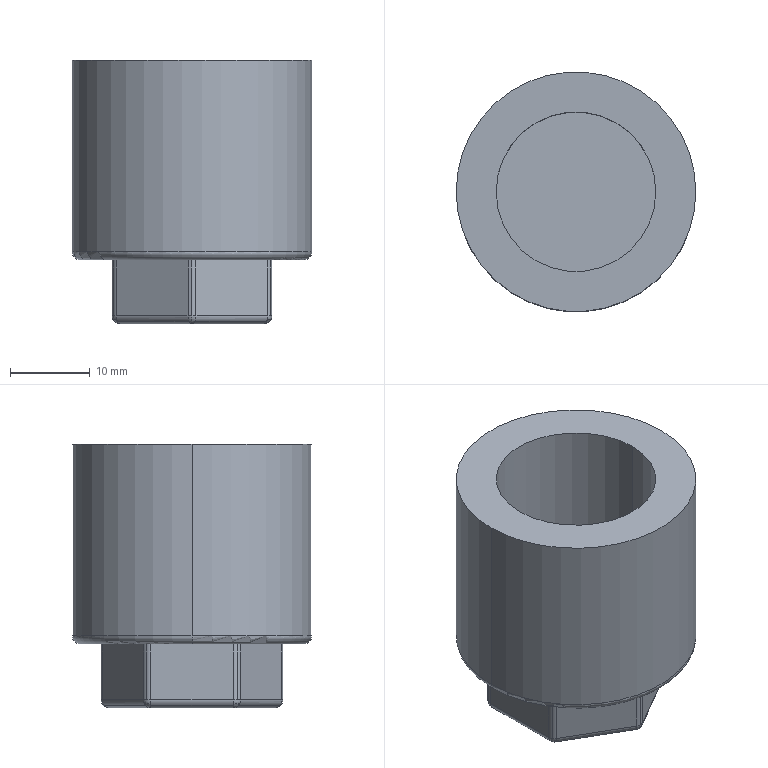Part | SolidWorks | features BaseBody 1 | 1 solid | 52 faces | box 30 x 30 x 33 mm | volume 14123 mm3 | cylinder 28 | sphere 12 | plane 10 | torus 2 | commonest cylinder face diameters 2 x24 20 x2 30 x2
STEP:
#1=CARTESIAN_POINT('',(0.,-10.392,-8.));
#2=VERTEX_POINT('',#1);
#3=CARTESIAN_POINT('',(-0.3536,-11.005,-7.707));
#4=VERTEX_POINT('',#3);
#5=CARTESIAN_POINT('',(0.,-10.392,-7.));
#6=DIRECTION('',(-0.866,0.5,0.));
#7=DIRECTION('',(0.,0.,-1.));
#8=AXIS2_PLACEMENT_3D('',#5,#6,#7);
#9=CIRCLE('',#8,1.);
#10=EDGE_CURVE('',#2,#4,#9,.T.);
#11=ORIENTED_EDGE('',*,*,#10,.F.);
#12=CARTESIAN_POINT('',(0.,-11.392,-7.));
#13=VERTEX_POINT('',#12);
#14=CARTESIAN_POINT('',(0.,-10.392,-7.));
#15=DIRECTION('',(-1.,0.,0.));
#16=DIRECTION('',(0.,-1.,0.));
#17=AXIS2_PLACEMENT_3D('',#14,#15,#16);
#18=CIRCLE('',#17,1.);
#19=EDGE_CURVE('',#2,#13,#18,.T.);
#20=ORIENTED_EDGE('',*,*,#19,.T.);
#21=CARTESIAN_POINT('',(-0.5,-11.258,-7.));
#22=VERTEX_POINT('',#21);
#23=CARTESIAN_POINT('',(0.,-10.392,-7.));
#24=DIRECTION('',(0.,0.,1.));
#25=DIRECTION('',(-0.5,-0.866,0.));
#26=AXIS2_PLACEMENT_3D('',#23,#24,#25);
#27=CIRCLE('',#26,1.);
#28=EDGE_CURVE('',#22,#13,#27,.T.);
#29=ORIENTED_EDGE('',*,*,#28,.F.);
#30=CARTESIAN_POINT('',(0.,-10.392,-7.));
#31=DIRECTION('',(-0.866,0.5,0.));
#32=DIRECTION('',(0.,0.,-1.));
#33=AXIS2_PLACEMENT_3D('',#30,#31,#32);
#34=CIRCLE('',#33,1.);
#35=EDGE_CURVE('',#4,#22,#34,.T.);
#36=ORIENTED_EDGE('',*,*,#35,.F.);
#37=EDGE_LOOP('',(#11,#20,#29,#36));
#38=FACE_OUTER_BOUND('',#37,.T.);
#39=CARTESIAN_POINT('',(0.,-10.392,-7.));
#40=DIRECTION('',(1.,0.,0.));
#41=DIRECTION('',(0.,-0.866,-0.5));
#42=AXIS2_PLACEMENT_3D('',#39,#40,#41);
#43=SPHERICAL_SURFACE('',#42,1.);
#44=ADVANCED_FACE('',(#38),#43,.T.);
#45=ORIENTED_EDGE('',*,*,#28,.T.);
#46=CARTESIAN_POINT('',(0.,-11.392,0.));
#47=VERTEX_POINT('',#46);
#48=CARTESIAN_POINT('',(0.,-11.392,0.));
#49=DIRECTION('',(0.,0.,1.));
#50=VECTOR('',#49,1000.);
#51=LINE('',#48,#50);
#52=EDGE_CURVE('',#13,#47,#51,.T.);
#53=ORIENTED_EDGE('',*,*,#52,.T.);
#54=CARTESIAN_POINT('',(-0.5,-11.258,0.));
#55=VERTEX_POINT('',#54);
#56=CARTESIAN_POINT('',(0.,-10.392,0.));
#57=DIRECTION('',(0.,0.,-1.));
#58=DIRECTION('',(0.,-1.,0.));
#59=AXIS2_PLACEMENT_3D('',#56,#57,#58);
#60=CIRCLE('',#59,1.);
#61=EDGE_CURVE('',#47,#55,#60,.T.);
#62=ORIENTED_EDGE('',*,*,#61,.T.);
#63=CARTESIAN_POINT('',(-0.5,-11.258,0.));
#64=DIRECTION('',(0.,0.,-1.));
#65=VECTOR('',#64,1000.);
#66=LINE('',#63,#65);
#67=EDGE_CURVE('',#55,#22,#66,.T.);
#68=ORIENTED_EDGE('',*,*,#67,.T.);
#69=EDGE_LOOP('',(#45,#53,#62,#68));
#70=FACE_OUTER_BOUND('',#69,.T.);
#71=CARTESIAN_POINT('',(0.,-10.392,0.));
#72=DIRECTION('',(0.,0.,1.));
#73=DIRECTION('',(0.,-1.,0.));
#74=AXIS2_PLACEMENT_3D('',#71,#72,#73);
#75=CYLINDRICAL_SURFACE('',#74,1.);
#76=ADVANCED_FACE('',(#70),#75,.T.);
#77=CARTESIAN_POINT('',(-9.447,-5.971,-7.447));
#78=VERTEX_POINT('',#77);
#79=CARTESIAN_POINT('',(-9.354,-5.809,-7.707));
#80=VERTEX_POINT('',#79);
#81=CARTESIAN_POINT('',(-9.,-5.196,-7.));
#82=DIRECTION('',(0.866,-0.5,0.));
#83=DIRECTION('',(-0.5,-0.866,0.));
#84=AXIS2_PLACEMENT_3D('',#81,#82,#83);
#85=CIRCLE('',#84,1.);
#86=EDGE_CURVE('',#78,#80,#85,.T.);
#87=ORIENTED_EDGE('',*,*,#86,.F.);
#88=CARTESIAN_POINT('',(-9.894,-5.196,-7.447));
#89=VERTEX_POINT('',#88);
#90=CARTESIAN_POINT('',(-9.,-5.196,-7.));
#91=DIRECTION('',(0.433,0.25,-0.866));
#92=DIRECTION('',(-0.8944,0.,-0.4472));
#93=AXIS2_PLACEMENT_3D('',#90,#91,#92);
#94=CIRCLE('',#93,1.);
#95=EDGE_CURVE('',#78,#89,#94,.T.);
#96=ORIENTED_EDGE('',*,*,#95,.T.);
#97=CARTESIAN_POINT('',(-9.707,-5.196,-7.707));
#98=VERTEX_POINT('',#97);
#99=CARTESIAN_POINT('',(-9.,-5.196,-7.));
#100=DIRECTION('',(0.,1.,0.));
#101=DIRECTION('',(0.,0.,-1.));
#102=AXIS2_PLACEMENT_3D('',#99,#100,#101);
#103=CIRCLE('',#102,1.);
#104=EDGE_CURVE('',#98,#89,#103,.T.);
#105=ORIENTED_EDGE('',*,*,#104,.F.);
#106=CARTESIAN_POINT('',(-9.,-5.196,-8.));
#107=VERTEX_POINT('',#106);
#108=CARTESIAN_POINT('',(-9.,-5.196,-7.));
#109=DIRECTION('',(0.,1.,0.));
#110=DIRECTION('',(0.,0.,-1.));
#111=AXIS2_PLACEMENT_3D('',#108,#109,#110);
#112=CIRCLE('',#111,1.);
#113=EDGE_CURVE('',#107,#98,#112,.T.);
#114=ORIENTED_EDGE('',*,*,#113,.F.);
#115=CARTESIAN_POINT('',(-9.,-5.196,-7.));
#116=DIRECTION('',(0.866,-0.5,0.));
#117=DIRECTION('',(-0.5,-0.866,0.));
#118=AXIS2_PLACEMENT_3D('',#115,#116,#117);
#119=CIRCLE('',#118,1.);
#120=EDGE_CURVE('',#80,#107,#119,.T.);
#121=ORIENTED_EDGE('',*,*,#120,.F.);
#122=EDGE_LOOP('',(#87,#96,#105,#114,#121));
#123=FACE_OUTER_BOUND('',#122,.T.);
#124=CARTESIAN_POINT('',(-9.,-5.196,-7.));
#125=DIRECTION('',(-0.433,-0.25,0.866));
#126=DIRECTION('',(-0.75,-0.433,-0.5));
#127=AXIS2_PLACEMENT_3D('',#124,#125,#126);
#128=SPHERICAL_SURFACE('',#127,1.);
#129=ADVANCED_FACE('',(#123),#128,.T.);
#130=CARTESIAN_POINT('',(-10.,-5.196,-7.));
#131=VERTEX_POINT('',#130);
#132=CARTESIAN_POINT('',(-9.866,-5.696,-7.));
#133=VERTEX_POINT('',#132);
#134=CARTESIAN_POINT('',(-9.,-5.196,-7.));
#135=DIRECTION('',(0.,0.,1.));
#136=DIRECTION('',(-1.,0.,0.));
#137=AXIS2_PLACEMENT_3D('',#134,#135,#136);
#138=CIRCLE('',#137,1.);
#139=EDGE_CURVE('',#131,#133,#138,.T.);
#140=ORIENTED_EDGE('',*,*,#139,.T.);
#141=CARTESIAN_POINT('',(-9.866,-5.696,0.));
#142=VERTEX_POINT('',#141);
#143=CARTESIAN_POINT('',(-9.866,-5.696,0.));
#144=DIRECTION('',(0.,0.,1.));
#145=VECTOR('',#144,1000.);
#146=LINE('',#143,#145);
#147=EDGE_CURVE('',#133,#142,#146,.T.);
#148=ORIENTED_EDGE('',*,*,#147,.T.);
#149=CARTESIAN_POINT('',(-10.,-5.196,0.));
#150=VERTEX_POINT('',#149);
#151=CARTESIAN_POINT('',(-9.,-5.196,0.));
#152=DIRECTION('',(0.,0.,-1.));
#153=DIRECTION('',(-0.866,-0.5,0.));
#154=AXIS2_PLACEMENT_3D('',#151,#152,#153);
#155=CIRCLE('',#154,1.);
#156=EDGE_CURVE('',#142,#150,#155,.T.);
#157=ORIENTED_EDGE('',*,*,#156,.T.);
#158=CARTESIAN_POINT('',(-10.,-5.196,0.));
#159=DIRECTION('',(0.,0.,-1.));
#160=VECTOR('',#159,1000.);
#161=LINE('',#158,#160);
#162=EDGE_CURVE('',#150,#131,#161,.T.);
#163=ORIENTED_EDGE('',*,*,#162,.T.);
#164=EDGE_LOOP('',(#140,#148,#157,#163));
#165=FACE_OUTER_BOUND('',#164,.T.);
#166=CARTESIAN_POINT('',(-9.,-5.196,0.));
#167=DIRECTION('',(0.,0.,1.));
#168=DIRECTION('',(-0.866,-0.5,0.));
#169=AXIS2_PLACEMENT_3D('',#166,#167,#168);
#170=CYLINDRICAL_SURFACE('',#169,1.);
#171=ADVANCED_FACE('',(#165),#170,.T.);
#172=CARTESIAN_POINT('',(9.894,-5.196,-7.447));
#173=VERTEX_POINT('',#172);
#174=CARTESIAN_POINT('',(9.707,-5.196,-7.707));
#175=VERTEX_POINT('',#174);
#176=CARTESIAN_POINT('',(9.,-5.196,-7.));
#177=DIRECTION('',(0.,1.,0.));
#178=DIRECTION('',(1.,0.,0.));
#179=AXIS2_PLACEMENT_3D('',#176,#177,#178);
#180=CIRCLE('',#179,1.);
#181=EDGE_CURVE('',#173,#175,#180,.T.);
#182=ORIENTED_EDGE('',*,*,#181,.F.);
#183=CARTESIAN_POINT('',(9.447,-5.971,-7.447));
#184=VERTEX_POINT('',#183);
#185=CARTESIAN_POINT('',(9.,-5.196,-7.));
#186=DIRECTION('',(-0.433,0.25,-0.866));
#187=DIRECTION('',(-0.8944,0.,0.4472));
#188=AXIS2_PLACEMENT_3D('',#185,#186,#187);
#189=CIRCLE('',#188,1.);
#190=EDGE_CURVE('',#173,#184,#189,.T.);
#191=ORIENTED_EDGE('',*,*,#190,.T.);
#192=CARTESIAN_POINT('',(9.354,-5.809,-7.707));
#193=VERTEX_POINT('',#192);
#194=CARTESIAN_POINT('',(9.,-5.196,-7.));
#195=DIRECTION('',(-0.866,-0.5,0.));
#196=DIRECTION('',(0.,0.,-1.));
#197=AXIS2_PLACEMENT_3D('',#194,#195,#196);
#198=CIRCLE('',#197,1.);
#199=EDGE_CURVE('',#193,#184,#198,.T.);
#200=ORIENTED_EDGE('',*,*,#199,.F.);
#201=CARTESIAN_POINT('',(9.,-5.196,-8.));
#202=VERTEX_POINT('',#201);
#203=CARTESIAN_POINT('',(9.,-5.196,-7.));
#204=DIRECTION('',(-0.866,-0.5,0.));
#205=DIRECTION('',(0.,0.,-1.));
#206=AXIS2_PLACEMENT_3D('',#203,#204,#205);
#207=CIRCLE('',#206,1.);
#208=EDGE_CURVE('',#202,#193,#207,.T.);
#209=ORIENTED_EDGE('',*,*,#208,.F.);
#210=CARTESIAN_POINT('',(9.,-5.196,-7.));
#211=DIRECTION('',(0.,1.,0.));
#212=DIRECTION('',(1.,0.,0.));
#213=AXIS2_PLACEMENT_3D('',#210,#211,#212);
#214=CIRCLE('',#213,1.);
#215=EDGE_CURVE('',#175,#202,#214,.T.);
#216=ORIENTED_EDGE('',*,*,#215,.F.);
#217=EDGE_LOOP('',(#182,#191,#200,#209,#216));
#218=FACE_OUTER_BOUND('',#217,.T.);
#219=CARTESIAN_POINT('',(9.,-5.196,-7.));
#220=DIRECTION('',(0.433,-0.25,0.866));
#221=DIRECTION('',(0.75,-0.433,-0.5));
#222=AXIS2_PLACEMENT_3D('',#219,#220,#221);
#223=SPHERICAL_SURFACE('',#222,1.);
#224=ADVANCED_FACE('',(#218),#223,.T.);
#225=CARTESIAN_POINT('',(9.5,-6.062,-7.));
#226=VERTEX_POINT('',#225);
#227=CARTESIAN_POINT('',(9.866,-5.696,-7.));
#228=VERTEX_POINT('',#227);
#229=CARTESIAN_POINT('',(9.,-5.196,-7.));
#230=DIRECTION('',(0.,0.,1.));
#231=DIRECTION('',(0.5,-0.866,0.));
#232=AXIS2_PLACEMENT_3D('',#229,#230,#231);
#233=CIRCLE('',#232,1.);
#234=EDGE_CURVE('',#226,#228,#233,.T.);
#235=ORIENTED_EDGE('',*,*,#234,.T.);
#236=CARTESIAN_POINT('',(9.866,-5.696,0.));
#237=VERTEX_POINT('',#236);
#238=CARTESIAN_POINT('',(9.866,-5.696,0.));
#239=DIRECTION('',(0.,0.,1.));
#240=VECTOR('',#239,1000.);
#241=LINE('',#238,#240);
#242=EDGE_CURVE('',#228,#237,#241,.T.);
#243=ORIENTED_EDGE('',*,*,#242,.T.);
#244=CARTESIAN_POINT('',(9.5,-6.062,0.));
#245=VERTEX_POINT('',#244);
#246=CARTESIAN_POINT('',(9.,-5.196,0.));
#247=DIRECTION('',(0.,0.,-1.));
#248=DIRECTION('',(0.866,-0.5,0.));
#249=AXIS2_PLACEMENT_3D('',#246,#247,#248);
#250=CIRCLE('',#249,1.);
#251=EDGE_CURVE('',#237,#245,#250,.T.);
#252=ORIENTED_EDGE('',*,*,#251,.T.);
#253=CARTESIAN_POINT('',(9.5,-6.062,0.));
#254=DIRECTION('',(0.,0.,-1.));
#255=VECTOR('',#254,1000.);
#256=LINE('',#253,#255);
#257=EDGE_CURVE('',#245,#226,#256,.T.);
#258=ORIENTED_EDGE('',*,*,#257,.T.);
#259=EDGE_LOOP('',(#235,#243,#252,#258));
#260=FACE_OUTER_BOUND('',#259,.T.);
#261=CARTESIAN_POINT('',(9.,-5.196,0.));
#262=DIRECTION('',(0.,0.,1.));
#263=DIRECTION('',(0.866,-0.5,0.));
#264=AXIS2_PLACEMENT_3D('',#261,#262,#263);
#265=CYLINDRICAL_SURFACE('',#264,1.);
#266=ADVANCED_FACE('',(#260),#265,.T.);
#267=CARTESIAN_POINT('',(0.5,-11.258,-7.));
#268=VERTEX_POINT('',#267);
#269=CARTESIAN_POINT('',(0.3536,-11.005,-7.707));
#270=VERTEX_POINT('',#269);
#271=CARTESIAN_POINT('',(0.,-10.392,-7.));
#272=DIRECTION('',(0.866,0.5,0.));
#273=DIRECTION('',(0.5,-0.866,0.));
#274=AXIS2_PLACEMENT_3D('',#271,#272,#273);
#275=CIRCLE('',#274,1.);
#276=EDGE_CURVE('',#268,#270,#275,.T.);
#277=ORIENTED_EDGE('',*,*,#276,.T.);
#278=CARTESIAN_POINT('',(7.354,-6.963,-7.707));
#279=DIRECTION('',(0.866,0.5,0.));
#280=VECTOR('',#279,1000.);
#281=LINE('',#278,#280);
#282=EDGE_CURVE('',#270,#193,#281,.T.);
#283=ORIENTED_EDGE('',*,*,#282,.T.);
#284=ORIENTED_EDGE('',*,*,#199,.T.);
#285=CARTESIAN_POINT('',(9.,-5.196,-7.));
#286=DIRECTION('',(-0.866,-0.5,0.));
#287=DIRECTION('',(0.,0.,-1.));
#288=AXIS2_PLACEMENT_3D('',#285,#286,#287);
#289=CIRCLE('',#288,1.);
#290=EDGE_CURVE('',#184,#226,#289,.T.);
#291=ORIENTED_EDGE('',*,*,#290,.T.);
#292=CARTESIAN_POINT('',(7.5,-7.217,-7.));
#293=DIRECTION('',(-0.866,-0.5,0.));
#294=VECTOR('',#293,1000.);
#295=LINE('',#292,#294);
#296=EDGE_CURVE('',#226,#268,#295,.T.);
#297=ORIENTED_EDGE('',*,*,#296,.T.);
#298=EDGE_LOOP('',(#277,#283,#284,#291,#297));
#299=FACE_OUTER_BOUND('',#298,.T.);
#300=CARTESIAN_POINT('',(7.,-6.351,-7.));
#301=DIRECTION('',(0.866,0.5,0.));
#302=DIRECTION('',(0.3536,-0.6124,-0.7071));
#303=AXIS2_PLACEMENT_3D('',#300,#301,#302);
#304=CYLINDRICAL_SURFACE('',#303,1.);
#305=ADVANCED_FACE('',(#299),#304,.T.);
#306=CARTESIAN_POINT('',(-9.894,5.196,-7.447));
#307=VERTEX_POINT('',#306);
#308=CARTESIAN_POINT('',(-9.707,5.196,-7.707));
#309=VERTEX_POINT('',#308);
#310=CARTESIAN_POINT('',(-9.,5.196,-7.));
#311=DIRECTION('',(0.,-1.,0.));
#312=DIRECTION('',(-1.,0.,0.));
#313=AXIS2_PLACEMENT_3D('',#310,#311,#312);
#314=CIRCLE('',#313,1.);
#315=EDGE_CURVE('',#307,#309,#314,.T.);
#316=ORIENTED_EDGE('',*,*,#315,.F.);
#317=CARTESIAN_POINT('',(-9.447,5.971,-7.447));
#318=VERTEX_POINT('',#317);
#319=CARTESIAN_POINT('',(-9.,5.196,-7.));
#320=DIRECTION('',(0.433,-0.25,-0.866));
#321=DIRECTION('',(-0.8944,0.,-0.4472));
#322=AXIS2_PLACEMENT_3D('',#319,#320,#321);
#323=CIRCLE('',#322,1.);
#324=EDGE_CURVE('',#307,#318,#323,.T.);
#325=ORIENTED_EDGE('',*,*,#324,.T.);
#326=CARTESIAN_POINT('',(-9.354,5.809,-7.707));
#327=VERTEX_POINT('',#326);
#328=CARTESIAN_POINT('',(-9.,5.196,-7.));
#329=DIRECTION('',(0.866,0.5,0.));
#330=DIRECTION('',(0.,0.,-1.));
#331=AXIS2_PLACEMENT_3D('',#328,#329,#330);
#332=CIRCLE('',#331,1.);
#333=EDGE_CURVE('',#327,#318,#332,.T.);
#334=ORIENTED_EDGE('',*,*,#333,.F.);
#335=CARTESIAN_POINT('',(-9.,5.196,-8.));
#336=VERTEX_POINT('',#335);
#337=CARTESIAN_POINT('',(-9.,5.196,-7.));
#338=DIRECTION('',(0.866,0.5,0.));
#339=DIRECTION('',(0.,0.,-1.));
#340=AXIS2_PLACEMENT_3D('',#337,#338,#339);
#341=CIRCLE('',#340,1.);
#342=EDGE_CURVE('',#336,#327,#341,.T.);
#343=ORIENTED_EDGE('',*,*,#342,.F.);
#344=CARTESIAN_POINT('',(-9.,5.196,-7.));
#345=DIRECTION('',(0.,-1.,0.));
#346=DIRECTION('',(-1.,0.,0.));
#347=AXIS2_PLACEMENT_3D('',#344,#345,#346);
#348=CIRCLE('',#347,1.);
#349=EDGE_CURVE('',#309,#336,#348,.T.);
#350=ORIENTED_EDGE('',*,*,#349,.F.);
#351=EDGE_LOOP('',(#316,#325,#334,#343,#350));
#352=FACE_OUTER_BOUND('',#351,.T.);
#353=CARTESIAN_POINT('',(-9.,5.196,-7.));
#354=DIRECTION('',(-0.433,0.25,0.866));
#355=DIRECTION('',(-0.75,0.433,-0.5));
#356=AXIS2_PLACEMENT_3D('',#353,#354,#355);
#357=SPHERICAL_SURFACE('',#356,1.);
#358=ADVANCED_FACE('',(#352),#357,.T.);
#359=CARTESIAN_POINT('',(-9.5,6.062,-7.));
#360=VERTEX_POINT('',#359);
#361=CARTESIAN_POINT('',(-9.866,5.696,-7.));
#362=VERTEX_POINT('',#361);
#363=CARTESIAN_POINT('',(-9.,5.196,-7.));
#364=DIRECTION('',(0.,0.,1.));
#365=DIRECTION('',(-0.5,0.866,0.));
#366=AXIS2_PLACEMENT_3D('',#363,#364,#365);
#367=CIRCLE('',#366,1.);
#368=EDGE_CURVE('',#360,#362,#367,.T.);
#369=ORIENTED_EDGE('',*,*,#368,.T.);
#370=CARTESIAN_POINT('',(-9.866,5.696,0.));
#371=VERTEX_POINT('',#370);
#372=CARTESIAN_POINT('',(-9.866,5.696,0.));
#373=DIRECTION('',(0.,0.,1.));
#374=VECTOR('',#373,1000.);
#375=LINE('',#372,#374);
#376=EDGE_CURVE('',#362,#371,#375,.T.);
#377=ORIENTED_EDGE('',*,*,#376,.T.);
#378=CARTESIAN_POINT('',(-9.5,6.062,0.));
#379=VERTEX_POINT('',#378);
#380=CARTESIAN_POINT('',(-9.,5.196,0.));
#381=DIRECTION('',(0.,0.,-1.));
#382=DIRECTION('',(-0.866,0.5,0.));
#383=AXIS2_PLACEMENT_3D('',#380,#381,#382);
#384=CIRCLE('',#383,1.);
#385=EDGE_CURVE('',#371,#379,#384,.T.);
#386=ORIENTED_EDGE('',*,*,#385,.T.);
#387=CARTESIAN_POINT('',(-9.5,6.062,0.));
#388=DIRECTION('',(0.,0.,-1.));
#389=VECTOR('',#388,1000.);
#390=LINE('',#387,#389);
#391=EDGE_CURVE('',#379,#360,#390,.T.);
#392=ORIENTED_EDGE('',*,*,#391,.T.);
#393=EDGE_LOOP('',(#369,#377,#386,#392));
#394=FACE_OUTER_BOUND('',#393,.T.);
#395=CARTESIAN_POINT('',(-9.,5.196,0.));
#396=DIRECTION('',(0.,0.,1.));
#397=DIRECTION('',(-0.866,0.5,0.));
#398=AXIS2_PLACEMENT_3D('',#395,#396,#397);
#399=CYLINDRICAL_SURFACE('',#398,1.);
#400=ADVANCED_FACE('',(#394),#399,.T.);
#401=CARTESIAN_POINT('',(9.447,5.971,-7.447));
#402=VERTEX_POINT('',#401);
#403=CARTESIAN_POINT('',(9.354,5.809,-7.707));
#404=VERTEX_POINT('',#403);
#405=CARTESIAN_POINT('',(9.,5.196,-7.));
#406=DIRECTION('',(-0.866,0.5,0.));
#407=DIRECTION('',(0.5,0.866,0.));
#408=AXIS2_PLACEMENT_3D('',#405,#406,#407);
#409=CIRCLE('',#408,1.);
#410=EDGE_CURVE('',#402,#404,#409,.T.);
#411=ORIENTED_EDGE('',*,*,#410,.F.);
#412=CARTESIAN_POINT('',(9.894,5.196,-7.447));
#413=VERTEX_POINT('',#412);
#414=CARTESIAN_POINT('',(9.,5.196,-7.));
#415=DIRECTION('',(-0.433,-0.25,-0.866));
#416=DIRECTION('',(-0.8944,0.,0.4472));
#417=AXIS2_PLACEMENT_3D('',#414,#415,#416);
#418=CIRCLE('',#417,1.);
#419=EDGE_CURVE('',#402,#413,#418,.T.);
#420=ORIENTED_EDGE('',*,*,#419,.T.);
#421=CARTESIAN_POINT('',(9.707,5.196,-7.707));
#422=VERTEX_POINT('',#421);
#423=CARTESIAN_POINT('',(9.,5.196,-7.));
#424=DIRECTION('',(0.,-1.,0.));
#425=DIRECTION('',(0.,0.,-1.));
#426=AXIS2_PLACEMENT_3D('',#423,#424,#425);
#427=CIRCLE('',#426,1.);
#428=EDGE_CURVE('',#422,#413,#427,.T.);
#429=ORIENTED_EDGE('',*,*,#428,.F.);
#430=CARTESIAN_POINT('',(9.,5.196,-8.));
#431=VERTEX_POINT('',#430);
#432=CARTESIAN_POINT('',(9.,5.196,-7.));
#433=DIRECTION('',(0.,-1.,0.));
#434=DIRECTION('',(0.,0.,-1.));
#435=AXIS2_PLACEMENT_3D('',#432,#433,#434);
#436=CIRCLE('',#435,1.);
#437=EDGE_CURVE('',#431,#422,#436,.T.);
#438=ORIENTED_EDGE('',*,*,#437,.F.);
#439=CARTESIAN_POINT('',(9.,5.196,-7.));
#440=DIRECTION('',(-0.866,0.5,0.));
#441=DIRECTION('',(0.5,0.866,0.));
#442=AXIS2_PLACEMENT_3D('',#439,#440,#441);
#443=CIRCLE('',#442,1.);
#444=EDGE_CURVE('',#404,#431,#443,.T.);
#445=ORIENTED_EDGE('',*,*,#444,.F.);
#446=EDGE_LOOP('',(#411,#420,#429,#438,#445));
#447=FACE_OUTER_BOUND('',#446,.T.);
#448=CARTESIAN_POINT('',(9.,5.196,-7.));
#449=DIRECTION('',(0.433,0.25,0.866));
#450=DIRECTION('',(0.75,0.433,-0.5));
#451=AXIS2_PLACEMENT_3D('',#448,#449,#450);
#452=SPHERICAL_SURFACE('',#451,1.);
#453=ADVANCED_FACE('',(#447),#452,.T.);
#454=CARTESIAN_POINT('',(10.,5.196,-7.));
#455=VERTEX_POINT('',#454);
#456=CARTESIAN_POINT('',(9.866,5.696,-7.));
#457=VERTEX_POINT('',#456);
#458=CARTESIAN_POINT('',(9.,5.196,-7.));
#459=DIRECTION('',(0.,0.,1.));
#460=DIRECTION('',(1.,0.,0.));
#461=AXIS2_PLACEMENT_3D('',#458,#459,#460);
#462=CIRCLE('',#461,1.);
#463=EDGE_CURVE('',#455,#457,#462,.T.);
#464=ORIENTED_EDGE('',*,*,#463,.T.);
#465=CARTESIAN_POINT('',(9.866,5.696,0.));
#466=VERTEX_POINT('',#465);
#467=CARTESIAN_POINT('',(9.866,5.696,0.));
#468=DIRECTION('',(0.,0.,1.));
#469=VECTOR('',#468,1000.);
#470=LINE('',#467,#469);
#471=EDGE_CURVE('',#457,#466,#470,.T.);
#472=ORIENTED_EDGE('',*,*,#471,.T.);
#473=CARTESIAN_POINT('',(10.,5.196,0.));
#474=VERTEX_POINT('',#473);
#475=CARTESIAN_POINT('',(9.,5.196,0.));
#476=DIRECTION('',(0.,0.,-1.));
#477=DIRECTION('',(0.866,0.5,0.));
#478=AXIS2_PLACEMENT_3D('',#475,#476,#477);
#479=CIRCLE('',#478,1.);
#480=EDGE_CURVE('',#466,#474,#479,.T.);
#481=ORIENTED_EDGE('',*,*,#480,.T.);
#482=CARTESIAN_POINT('',(10.,5.196,0.));
#483=DIRECTION('',(0.,0.,-1.));
#484=VECTOR('',#483,1000.);
#485=LINE('',#482,#484);
#486=EDGE_CURVE('',#474,#455,#485,.T.);
#487=ORIENTED_EDGE('',*,*,#486,.T.);
#488=EDGE_LOOP('',(#464,#472,#481,#487));
#489=FACE_OUTER_BOUND('',#488,.T.);
#490=CARTESIAN_POINT('',(9.,5.196,0.));
#491=DIRECTION('',(0.,0.,1.));
#492=DIRECTION('',(0.866,0.5,0.));
#493=AXIS2_PLACEMENT_3D('',#490,#491,#492);
#494=CYLINDRICAL_SURFACE('',#493,1.);
#495=ADVANCED_FACE('',(#489),#494,.T.);
#496=CARTESIAN_POINT('',(10.,-5.196,-7.));
#497=VERTEX_POINT('',#496);
#498=CARTESIAN_POINT('',(9.,-5.196,-7.));
#499=DIRECTION('',(0.,1.,0.));
#500=DIRECTION('',(1.,0.,0.));
#501=AXIS2_PLACEMENT_3D('',#498,#499,#500);
#502=CIRCLE('',#501,1.);
#503=EDGE_CURVE('',#497,#173,#502,.T.);
#504=ORIENTED_EDGE('',*,*,#503,.T.);
#505=ORIENTED_EDGE('',*,*,#181,.T.);
#506=CARTESIAN_POINT('',(9.707,2.887,-7.707));
#507=DIRECTION('',(0.,1.,0.));
#508=VECTOR('',#507,1000.);
#509=LINE('',#506,#508);
#510=EDGE_CURVE('',#175,#422,#509,.T.);
#511=ORIENTED_EDGE('',*,*,#510,.T.);
#512=ORIENTED_EDGE('',*,*,#428,.T.);
#513=CARTESIAN_POINT('',(9.,5.196,-7.));
#514=DIRECTION('',(0.,-1.,0.));
#515=DIRECTION('',(0.,0.,-1.));
#516=AXIS2_PLACEMENT_3D('',#513,#514,#515);
#517=CIRCLE('',#516,1.);
#518=EDGE_CURVE('',#413,#455,#517,.T.);
#519=ORIENTED_EDGE('',*,*,#518,.T.);
#520=CARTESIAN_POINT('',(10.,2.887,-7.));
#521=DIRECTION('',(0.,-1.,0.));
#522=VECTOR('',#521,1000.);
#523=LINE('',#520,#522);
#524=EDGE_CURVE('',#455,#497,#523,.T.);
#525=ORIENTED_EDGE('',*,*,#524,.T.);
#526=EDGE_LOOP('',(#504,#505,#511,#512,#519,#525));
#527=FACE_OUTER_BOUND('',#526,.T.);
#528=CARTESIAN_POINT('',(9.,2.887,-7.));
#529=DIRECTION('',(0.,1.,0.));
#530=DIRECTION('',(0.7071,0.,-0.7071));
#531=AXIS2_PLACEMENT_3D('',#528,#529,#530);
#532=CYLINDRICAL_SURFACE('',#531,1.);
#533=ADVANCED_FACE('',(#527),#532,.T.);
#534=CARTESIAN_POINT('',(0.,11.392,-7.));
#535=VERTEX_POINT('',#534);
#536=CARTESIAN_POINT('',(-0.5,11.258,-7.));
#537=VERTEX_POINT('',#536);
#538=CARTESIAN_POINT('',(0.,10.392,-7.));
#539=DIRECTION('',(0.,0.,1.));
#540=DIRECTION('',(0.5,0.866,0.));
#541=AXIS2_PLACEMENT_3D('',#538,#539,#540);
#542=CIRCLE('',#541,1.);
#543=EDGE_CURVE('',#535,#537,#542,.T.);
#544=ORIENTED_EDGE('',*,*,#543,.F.);
#545=CARTESIAN_POINT('',(0.,10.392,-8.));
#546=VERTEX_POINT('',#545);
#547=CARTESIAN_POINT('',(0.,10.392,-7.));
#548=DIRECTION('',(-1.,0.,0.));
#549=DIRECTION('',(0.,-1.,0.));
#550=AXIS2_PLACEMENT_3D('',#547,#548,#549);
#551=CIRCLE('',#550,1.);
#552=EDGE_CURVE('',#535,#546,#551,.T.);
#553=ORIENTED_EDGE('',*,*,#552,.T.);
#554=CARTESIAN_POINT('',(-0.3536,11.005,-7.707));
#555=VERTEX_POINT('',#554);
#556=CARTESIAN_POINT('',(0.,10.392,-7.));
#557=DIRECTION('',(-0.866,-0.5,0.));
#558=DIRECTION('',(-0.5,0.866,0.));
#559=AXIS2_PLACEMENT_3D('',#556,#557,#558);
#560=CIRCLE('',#559,1.);
#561=EDGE_CURVE('',#555,#546,#560,.T.);
#562=ORIENTED_EDGE('',*,*,#561,.F.);
#563=CARTESIAN_POINT('',(0.,10.392,-7.));
#564=DIRECTION('',(-0.866,-0.5,0.));
#565=DIRECTION('',(-0.5,0.866,0.));
#566=AXIS2_PLACEMENT_3D('',#563,#564,#565);
#567=CIRCLE('',#566,1.);
#568=EDGE_CURVE('',#537,#555,#567,.T.);
#569=ORIENTED_EDGE('',*,*,#568,.F.);
#570=EDGE_LOOP('',(#544,#553,#562,#569));
#571=FACE_OUTER_BOUND('',#570,.T.);
#572=CARTESIAN_POINT('',(0.,10.392,-7.));
#573=DIRECTION('',(1.,0.,0.));
#574=DIRECTION('',(0.,0.866,-0.5));
#575=AXIS2_PLACEMENT_3D('',#572,#573,#574);
#576=SPHERICAL_SURFACE('',#575,1.);
#577=ADVANCED_FACE('',(#571),#576,.T.);
#578=CARTESIAN_POINT('',(0.5,11.258,-7.));
#579=VERTEX_POINT('',#578);
#580=CARTESIAN_POINT('',(0.,10.392,-7.));
#581=DIRECTION('',(0.,0.,1.));
#582=DIRECTION('',(0.5,0.866,0.));
#583=AXIS2_PLACEMENT_3D('',#580,#581,#582);
#584=CIRCLE('',#583,1.);
#585=EDGE_CURVE('',#579,#535,#584,.T.);
#586=ORIENTED_EDGE('',*,*,#585,.T.);
#587=CARTESIAN_POINT('',(0.,11.392,0.));
#588=VERTEX_POINT('',#587);
#589=CARTESIAN_POINT('',(0.,11.392,0.));
#590=DIRECTION('',(0.,0.,1.));
#591=VECTOR('',#590,1000.);
#592=LINE('',#589,#591);
#593=EDGE_CURVE('',#535,#588,#592,.T.);
#594=ORIENTED_EDGE('',*,*,#593,.T.);
#595=CARTESIAN_POINT('',(0.5,11.258,0.));
#596=VERTEX_POINT('',#595);
#597=CARTESIAN_POINT('',(0.,10.392,0.));
#598=DIRECTION('',(0.,0.,-1.));
#599=DIRECTION('',(0.,1.,0.));
#600=AXIS2_PLACEMENT_3D('',#597,#598,#599);
#601=CIRCLE('',#600,1.);
#602=EDGE_CURVE('',#588,#596,#601,.T.);
#603=ORIENTED_EDGE('',*,*,#602,.T.);
#604=CARTESIAN_POINT('',(0.5,11.258,0.));
#605=DIRECTION('',(0.,0.,-1.));
#606=VECTOR('',#605,1000.);
#607=LINE('',#604,#606);
#608=EDGE_CURVE('',#596,#579,#607,.T.);
#609=ORIENTED_EDGE('',*,*,#608,.T.);
#610=EDGE_LOOP('',(#586,#594,#603,#609));
#611=FACE_OUTER_BOUND('',#610,.T.);
#612=CARTESIAN_POINT('',(0.,10.392,0.));
#613=DIRECTION('',(0.,0.,1.));
#614=DIRECTION('',(0.,1.,0.));
#615=AXIS2_PLACEMENT_3D('',#612,#613,#614);
#616=CYLINDRICAL_SURFACE('',#615,1.);
#617=ADVANCED_FACE('',(#611),#616,.T.);
#618=CARTESIAN_POINT('',(9.5,6.062,-7.));
#619=VERTEX_POINT('',#618);
#620=CARTESIAN_POINT('',(9.,5.196,-7.));
#621=DIRECTION('',(-0.866,0.5,0.));
#622=DIRECTION('',(0.5,0.866,0.));
#623=AXIS2_PLACEMENT_3D('',#620,#621,#622);
#624=CIRCLE('',#623,1.);
#625=EDGE_CURVE('',#619,#402,#624,.T.);
#626=ORIENTED_EDGE('',*,*,#625,.T.);
#627=ORIENTED_EDGE('',*,*,#410,.T.);
#628=CARTESIAN_POINT('',(0.3536,11.005,-7.707));
#629=VERTEX_POINT('',#628);
#630=CARTESIAN_POINT('',(2.354,9.85,-7.707));
#631=DIRECTION('',(-0.866,0.5,0.));
#632=VECTOR('',#631,1000.);
#633=LINE('',#630,#632);
#634=EDGE_CURVE('',#404,#629,#633,.T.);
#635=ORIENTED_EDGE('',*,*,#634,.T.);
#636=CARTESIAN_POINT('',(0.,10.392,-7.));
#637=DIRECTION('',(0.866,-0.5,0.));
#638=DIRECTION('',(0.,0.,-1.));
#639=AXIS2_PLACEMENT_3D('',#636,#637,#638);
#640=CIRCLE('',#639,1.);
#641=EDGE_CURVE('',#629,#579,#640,.T.);
#642=ORIENTED_EDGE('',*,*,#641,.T.);
#643=CARTESIAN_POINT('',(2.5,10.104,-7.));
#644=DIRECTION('',(0.866,-0.5,0.));
#645=VECTOR('',#644,1000.);
#646=LINE('',#643,#645);
#647=EDGE_CURVE('',#579,#619,#646,.T.);
#648=ORIENTED_EDGE('',*,*,#647,.T.);
#649=EDGE_LOOP('',(#626,#627,#635,#642,#648));
#650=FACE_OUTER_BOUND('',#649,.T.);
#651=CARTESIAN_POINT('',(2.,9.238,-7.));
#652=DIRECTION('',(-0.866,0.5,0.));
#653=DIRECTION('',(0.3536,0.6124,-0.7071));
#654=AXIS2_PLACEMENT_3D('',#651,#652,#653);
#655=CYLINDRICAL_SURFACE('',#654,1.);
#656=ADVANCED_FACE('',(#650),#655,.T.);
#657=ORIENTED_EDGE('',*,*,#568,.T.);
#658=CARTESIAN_POINT('',(-7.354,6.963,-7.707));
#659=DIRECTION('',(-0.866,-0.5,0.));
#660=VECTOR('',#659,1000.);
#661=LINE('',#658,#660);
#662=EDGE_CURVE('',#555,#327,#661,.T.);
#663=ORIENTED_EDGE('',*,*,#662,.T.);
#664=ORIENTED_EDGE('',*,*,#333,.T.);
#665=CARTESIAN_POINT('',(-9.,5.196,-7.));
#666=DIRECTION('',(0.866,0.5,0.));
#667=DIRECTION('',(0.,0.,-1.));
#668=AXIS2_PLACEMENT_3D('',#665,#666,#667);
#669=CIRCLE('',#668,1.);
#670=EDGE_CURVE('',#318,#360,#669,.T.);
#671=ORIENTED_EDGE('',*,*,#670,.T.);
#672=CARTESIAN_POINT('',(-7.5,7.217,-7.));
#673=DIRECTION('',(0.866,0.5,0.));
#674=VECTOR('',#673,1000.);
#675=LINE('',#672,#674);
#676=EDGE_CURVE('',#360,#537,#675,.T.);
#677=ORIENTED_EDGE('',*,*,#676,.T.);
#678=EDGE_LOOP('',(#657,#663,#664,#671,#677));
#679=FACE_OUTER_BOUND('',#678,.T.);
#680=CARTESIAN_POINT('',(-7.,6.351,-7.));
#681=DIRECTION('',(-0.866,-0.5,0.));
#682=DIRECTION('',(-0.3536,0.6124,-0.7071));
#683=AXIS2_PLACEMENT_3D('',#680,#681,#682);
#684=CYLINDRICAL_SURFACE('',#683,1.);
#685=ADVANCED_FACE('',(#679),#684,.T.);
#686=CARTESIAN_POINT('',(-10.,5.196,-7.));
#687=VERTEX_POINT('',#686);
#688=CARTESIAN_POINT('',(-9.,5.196,-7.));
#689=DIRECTION('',(0.,-1.,0.));
#690=DIRECTION('',(-1.,0.,0.));
#691=AXIS2_PLACEMENT_3D('',#688,#689,#690);
#692=CIRCLE('',#691,1.);
#693=EDGE_CURVE('',#687,#307,#692,.T.);
#694=ORIENTED_EDGE('',*,*,#693,.T.);
#695=ORIENTED_EDGE('',*,*,#315,.T.);
#696=CARTESIAN_POINT('',(-9.707,-2.887,-7.707));
#697=DIRECTION('',(0.,-1.,0.));
#698=VECTOR('',#697,1000.);
#699=LINE('',#696,#698);
#700=EDGE_CURVE('',#309,#98,#699,.T.);
#701=ORIENTED_EDGE('',*,*,#700,.T.);
#702=ORIENTED_EDGE('',*,*,#104,.T.);
#703=CARTESIAN_POINT('',(-9.,-5.196,-7.));
#704=DIRECTION('',(0.,1.,0.));
#705=DIRECTION('',(0.,0.,-1.));
#706=AXIS2_PLACEMENT_3D('',#703,#704,#705);
#707=CIRCLE('',#706,1.);
#708=EDGE_CURVE('',#89,#131,#707,.T.);
#709=ORIENTED_EDGE('',*,*,#708,.T.);
#710=CARTESIAN_POINT('',(-10.,-2.887,-7.));
#711=DIRECTION('',(0.,1.,0.));
#712=VECTOR('',#711,1000.);
#713=LINE('',#710,#712);
#714=EDGE_CURVE('',#131,#687,#713,.T.);
#715=ORIENTED_EDGE('',*,*,#714,.T.);
#716=EDGE_LOOP('',(#694,#695,#701,#702,#709,#715));
#717=FACE_OUTER_BOUND('',#716,.T.);
#718=CARTESIAN_POINT('',(-9.,-2.887,-7.));
#719=DIRECTION('',(0.,-1.,0.));
#720=DIRECTION('',(-0.7071,0.,-0.7071));
#721=AXIS2_PLACEMENT_3D('',#718,#719,#720);
#722=CYLINDRICAL_SURFACE('',#721,1.);
#723=ADVANCED_FACE('',(#717),#722,.T.);
#724=CARTESIAN_POINT('',(-9.5,-6.062,-7.));
#725=VERTEX_POINT('',#724);
#726=CARTESIAN_POINT('',(-9.,-5.196,-7.));
#727=DIRECTION('',(0.866,-0.5,0.));
#728=DIRECTION('',(-0.5,-0.866,0.));
#729=AXIS2_PLACEMENT_3D('',#726,#727,#728);
#730=CIRCLE('',#729,1.);
#731=EDGE_CURVE('',#725,#78,#730,.T.);
#732=ORIENTED_EDGE('',*,*,#731,.T.);
#733=ORIENTED_EDGE('',*,*,#86,.T.);
#734=CARTESIAN_POINT('',(-2.354,-9.85,-7.707));
#735=DIRECTION('',(0.866,-0.5,0.));
#736=VECTOR('',#735,1000.);
#737=LINE('',#734,#736);
#738=EDGE_CURVE('',#80,#4,#737,.T.);
#739=ORIENTED_EDGE('',*,*,#738,.T.);
#740=ORIENTED_EDGE('',*,*,#35,.T.);
#741=CARTESIAN_POINT('',(-2.5,-10.104,-7.));
#742=DIRECTION('',(-0.866,0.5,0.));
#743=VECTOR('',#742,1000.);
#744=LINE('',#741,#743);
#745=EDGE_CURVE('',#22,#725,#744,.T.);
#746=ORIENTED_EDGE('',*,*,#745,.T.);
#747=EDGE_LOOP('',(#732,#733,#739,#740,#746));
#748=FACE_OUTER_BOUND('',#747,.T.);
#749=CARTESIAN_POINT('',(-2.,-9.238,-7.));
#750=DIRECTION('',(0.866,-0.5,0.));
#751=DIRECTION('',(-0.3536,-0.6124,-0.7071));
#752=AXIS2_PLACEMENT_3D('',#749,#750,#751);
#753=CYLINDRICAL_SURFACE('',#752,1.);
#754=ADVANCED_FACE('',(#748),#753,.T.);
#755=CARTESIAN_POINT('',(-15.,0.,1.));
#756=VERTEX_POINT('',#755);
#757=CARTESIAN_POINT('',(15.,0.,1.));
#758=VERTEX_POINT('',#757);
#759=CARTESIAN_POINT('',(0.,0.,1.));
#760=DIRECTION('',(0.,0.,-1.));
#761=DIRECTION('',(-1.,0.,0.));
#762=AXIS2_PLACEMENT_3D('',#759,#760,#761);
#763=CIRCLE('',#762,15.);
#764=EDGE_CURVE('',#756,#758,#763,.T.);
#765=ORIENTED_EDGE('',*,*,#764,.T.);
#766=CARTESIAN_POINT('',(14.,0.,0.));
#767=VERTEX_POINT('',#766);
#768=CARTESIAN_POINT('',(14.,0.,1.));
#769=DIRECTION('',(0.,1.,0.));
#770=DIRECTION('',(-1.,0.,0.));
#771=AXIS2_PLACEMENT_3D('',#768,#769,#770);
#772=CIRCLE('',#771,1.);
#773=EDGE_CURVE('',#758,#767,#772,.T.);
#774=ORIENTED_EDGE('',*,*,#773,.T.);
#775=CARTESIAN_POINT('',(-14.,0.,0.));
#776=VERTEX_POINT('',#775);
#777=CARTESIAN_POINT('',(0.,0.,0.));
#778=DIRECTION('',(0.,0.,1.));
#779=DIRECTION('',(-1.,0.,0.));
#780=AXIS2_PLACEMENT_3D('',#777,#778,#779);
#781=CIRCLE('',#780,14.);
#782=EDGE_CURVE('',#767,#776,#781,.T.);
#783=ORIENTED_EDGE('',*,*,#782,.T.);
#784=CARTESIAN_POINT('',(-14.,0.,1.));
#785=DIRECTION('',(0.,-1.,0.));
#786=DIRECTION('',(0.,0.,-1.));
#787=AXIS2_PLACEMENT_3D('',#784,#785,#786);
#788=CIRCLE('',#787,1.);
#789=EDGE_CURVE('',#756,#776,#788,.T.);
#790=ORIENTED_EDGE('',*,*,#789,.F.);
#791=EDGE_LOOP('',(#765,#774,#783,#790));
#792=FACE_OUTER_BOUND('',#791,.T.);
#793=CARTESIAN_POINT('',(0.,0.,1.));
#794=DIRECTION('',(0.,0.,-1.));
#795=DIRECTION('',(-1.,0.,0.));
#796=AXIS2_PLACEMENT_3D('',#793,#794,#795);
#797=TOROIDAL_SURFACE('',#796,14.,1.);
#798=ADVANCED_FACE('',(#792),#797,.T.);
#799=CARTESIAN_POINT('',(15.,0.,25.));
#800=VERTEX_POINT('',#799);
#801=CARTESIAN_POINT('',(-15.,0.,25.));
#802=VERTEX_POINT('',#801);
#803=CARTESIAN_POINT('',(0.,0.,25.));
#804=DIRECTION('',(0.,0.,1.));
#805=DIRECTION('',(-1.,0.,0.));
#806=AXIS2_PLACEMENT_3D('',#803,#804,#805);
#807=CIRCLE('',#806,15.);
#808=EDGE_CURVE('',#800,#802,#807,.T.);
#809=ORIENTED_EDGE('',*,*,#808,.F.);
#810=CARTESIAN_POINT('',(15.,0.,0.));
#811=DIRECTION('',(0.,0.,-1.));
#812=VECTOR('',#811,1000.);
#813=LINE('',#810,#812);
#814=EDGE_CURVE('',#800,#758,#813,.T.);
#815=ORIENTED_EDGE('',*,*,#814,.T.);
#816=ORIENTED_EDGE('',*,*,#764,.F.);
#817=CARTESIAN_POINT('',(-15.,0.,0.));
#818=DIRECTION('',(0.,0.,-1.));
#819=VECTOR('',#818,1000.);
#820=LINE('',#817,#819);
#821=EDGE_CURVE('',#802,#756,#820,.T.);
#822=ORIENTED_EDGE('',*,*,#821,.F.);
#823=EDGE_LOOP('',(#809,#815,#816,#822));
#824=FACE_OUTER_BOUND('',#823,.T.);
#825=CARTESIAN_POINT('',(0.,0.,0.));
#826=DIRECTION('',(0.,0.,-1.));
#827=DIRECTION('',(-1.,0.,0.));
#828=AXIS2_PLACEMENT_3D('',#825,#826,#827);
#829=CYLINDRICAL_SURFACE('',#828,15.);
#830=ADVANCED_FACE('',(#824),#829,.T.);
#831=CARTESIAN_POINT('',(-10.,0.,5.));
#832=VERTEX_POINT('',#831);
#833=CARTESIAN_POINT('',(10.,0.,5.));
#834=VERTEX_POINT('',#833);
#835=CARTESIAN_POINT('',(0.,0.,5.));
#836=DIRECTION('',(0.,0.,-1.));
#837=DIRECTION('',(-1.,0.,0.));
#838=AXIS2_PLACEMENT_3D('',#835,#836,#837);
#839=CIRCLE('',#838,10.);
#840=EDGE_CURVE('',#832,#834,#839,.T.);
#841=ORIENTED_EDGE('',*,*,#840,.T.);
#842=CARTESIAN_POINT('',(10.,0.,25.));
#843=VERTEX_POINT('',#842);
#844=CARTESIAN_POINT('',(10.,0.,25.));
#845=DIRECTION('',(0.,0.,1.));
#846=VECTOR('',#845,1000.);
#847=LINE('',#844,#846);
#848=EDGE_CURVE('',#834,#843,#847,.T.);
#849=ORIENTED_EDGE('',*,*,#848,.T.);
#850=CARTESIAN_POINT('',(-10.,0.,25.));
#851=VERTEX_POINT('',#850);
#852=CARTESIAN_POINT('',(0.,0.,25.));
#853=DIRECTION('',(0.,0.,-1.));
#854=DIRECTION('',(-1.,0.,0.));
#855=AXIS2_PLACEMENT_3D('',#852,#853,#854);
#856=CIRCLE('',#855,10.);
#857=EDGE_CURVE('',#851,#843,#856,.T.);
#858=ORIENTED_EDGE('',*,*,#857,.F.);
#859=CARTESIAN_POINT('',(-10.,0.,25.));
#860=DIRECTION('',(0.,0.,1.));
#861=VECTOR('',#860,1000.);
#862=LINE('',#859,#861);
#863=EDGE_CURVE('',#832,#851,#862,.T.);
#864=ORIENTED_EDGE('',*,*,#863,.F.);
#865=EDGE_LOOP('',(#841,#849,#858,#864));
#866=FACE_OUTER_BOUND('',#865,.T.);
#867=CARTESIAN_POINT('',(0.,0.,25.));
#868=DIRECTION('',(0.,0.,1.));
#869=DIRECTION('',(-1.,0.,0.));
#870=AXIS2_PLACEMENT_3D('',#867,#868,#869);
#871=CYLINDRICAL_SURFACE('',#870,10.);
#872=ADVANCED_FACE('',(#866),#871,.F.);
#873=CARTESIAN_POINT('',(0.5,-11.258,0.));
#874=VERTEX_POINT('',#873);
#875=CARTESIAN_POINT('',(0.5,-11.258,0.));
#876=DIRECTION('',(0.,0.,1.));
#877=VECTOR('',#876,1000.);
#878=LINE('',#875,#877);
#879=EDGE_CURVE('',#268,#874,#878,.T.);
#880=ORIENTED_EDGE('',*,*,#879,.F.);
#881=ORIENTED_EDGE('',*,*,#296,.F.);
#882=ORIENTED_EDGE('',*,*,#257,.F.);
#883=CARTESIAN_POINT('',(7.5,-7.217,0.));
#884=DIRECTION('',(0.866,0.5,0.));
#885=VECTOR('',#884,1000.);
#886=LINE('',#883,#885);
#887=EDGE_CURVE('',#874,#245,#886,.T.);
#888=ORIENTED_EDGE('',*,*,#887,.F.);
#889=EDGE_LOOP('',(#880,#881,#882,#888));
#890=FACE_OUTER_BOUND('',#889,.T.);
#891=CARTESIAN_POINT('',(10.,-5.774,0.));
#892=DIRECTION('',(0.5,-0.866,0.));
#893=DIRECTION('',(0.,0.,-1.));
#894=AXIS2_PLACEMENT_3D('',#891,#892,#893);
#895=PLANE('',#894);
#896=ADVANCED_FACE('',(#890),#895,.T.);
#897=CARTESIAN_POINT('',(10.,-5.196,0.));
#898=VERTEX_POINT('',#897);
#899=CARTESIAN_POINT('',(10.,-5.196,0.));
#900=DIRECTION('',(0.,0.,1.));
#901=VECTOR('',#900,1000.);
#902=LINE('',#899,#901);
#903=EDGE_CURVE('',#497,#898,#902,.T.);
#904=ORIENTED_EDGE('',*,*,#903,.F.);
#905=ORIENTED_EDGE('',*,*,#524,.F.);
#906=ORIENTED_EDGE('',*,*,#486,.F.);
#907=CARTESIAN_POINT('',(10.,2.887,0.));
#908=DIRECTION('',(0.,1.,0.));
#909=VECTOR('',#908,1000.);
#910=LINE('',#907,#909);
#911=EDGE_CURVE('',#898,#474,#910,.T.);
#912=ORIENTED_EDGE('',*,*,#911,.F.);
#913=EDGE_LOOP('',(#904,#905,#906,#912));
#914=FACE_OUTER_BOUND('',#913,.T.);
#915=CARTESIAN_POINT('',(10.,5.774,0.));
#916=DIRECTION('',(1.,0.,0.));
#917=DIRECTION('',(0.,-1.,0.));
#918=AXIS2_PLACEMENT_3D('',#915,#916,#917);
#919=PLANE('',#918);
#920=ADVANCED_FACE('',(#914),#919,.T.);
#921=CARTESIAN_POINT('',(9.5,6.062,0.));
#922=VERTEX_POINT('',#921);
#923=CARTESIAN_POINT('',(9.5,6.062,0.));
#924=DIRECTION('',(0.,0.,1.));
#925=VECTOR('',#924,1000.);
#926=LINE('',#923,#925);
#927=EDGE_CURVE('',#619,#922,#926,.T.);
#928=ORIENTED_EDGE('',*,*,#927,.F.);
#929=ORIENTED_EDGE('',*,*,#647,.F.);
#930=ORIENTED_EDGE('',*,*,#608,.F.);
#931=CARTESIAN_POINT('',(2.5,10.104,0.));
#932=DIRECTION('',(-0.866,0.5,0.));
#933=VECTOR('',#932,1000.);
#934=LINE('',#931,#933);
#935=EDGE_CURVE('',#922,#596,#934,.T.);
#936=ORIENTED_EDGE('',*,*,#935,.F.);
#937=EDGE_LOOP('',(#928,#929,#930,#936));
#938=FACE_OUTER_BOUND('',#937,.T.);
#939=CARTESIAN_POINT('',(0.,11.547,0.));
#940=DIRECTION('',(0.5,0.866,0.));
#941=DIRECTION('',(0.,0.,-1.));
#942=AXIS2_PLACEMENT_3D('',#939,#940,#941);
#943=PLANE('',#942);
#944=ADVANCED_FACE('',(#938),#943,.T.);
#945=CARTESIAN_POINT('',(7.,-6.351,-8.));
#946=DIRECTION('',(0.866,0.5,0.));
#947=VECTOR('',#946,1000.);
#948=LINE('',#945,#947);
#949=EDGE_CURVE('',#2,#202,#948,.T.);
#950=ORIENTED_EDGE('',*,*,#949,.F.);
#951=CARTESIAN_POINT('',(-2.,-9.238,-8.));
#952=DIRECTION('',(0.866,-0.5,0.));
#953=VECTOR('',#952,1000.);
#954=LINE('',#951,#953);
#955=EDGE_CURVE('',#107,#2,#954,.T.);
#956=ORIENTED_EDGE('',*,*,#955,.F.);
#957=CARTESIAN_POINT('',(-9.,-2.887,-8.));
#958=DIRECTION('',(0.,-1.,0.));
#959=VECTOR('',#958,1000.);
#960=LINE('',#957,#959);
#961=EDGE_CURVE('',#336,#107,#960,.T.);
#962=ORIENTED_EDGE('',*,*,#961,.F.);
#963=CARTESIAN_POINT('',(-7.,6.351,-8.));
#964=DIRECTION('',(-0.866,-0.5,0.));
#965=VECTOR('',#964,1000.);
#966=LINE('',#963,#965);
#967=EDGE_CURVE('',#546,#336,#966,.T.);
#968=ORIENTED_EDGE('',*,*,#967,.F.);
#969=CARTESIAN_POINT('',(2.,9.238,-8.));
#970=DIRECTION('',(-0.866,0.5,0.));
#971=VECTOR('',#970,1000.);
#972=LINE('',#969,#971);
#973=EDGE_CURVE('',#431,#546,#972,.T.);
#974=ORIENTED_EDGE('',*,*,#973,.F.);
#975=CARTESIAN_POINT('',(9.,2.887,-8.));
#976=DIRECTION('',(0.,1.,0.));
#977=VECTOR('',#976,1000.);
#978=LINE('',#975,#977);
#979=EDGE_CURVE('',#202,#431,#978,.T.);
#980=ORIENTED_EDGE('',*,*,#979,.F.);
#981=EDGE_LOOP('',(#950,#956,#962,#968,#974,#980));
#982=FACE_OUTER_BOUND('',#981,.T.);
#983=CARTESIAN_POINT('',(0.,0.,-8.));
#984=DIRECTION('',(0.,0.,-1.));
#985=DIRECTION('',(0.,-1.,0.));
#986=AXIS2_PLACEMENT_3D('',#983,#984,#985);
#987=PLANE('',#986);
#988=ADVANCED_FACE('',(#982),#987,.T.);
#989=CARTESIAN_POINT('',(-9.5,-6.062,0.));
#990=VERTEX_POINT('',#989);
#991=CARTESIAN_POINT('',(-2.5,-10.104,0.));
#992=DIRECTION('',(0.866,-0.5,0.));
#993=VECTOR('',#992,1000.);
#994=LINE('',#991,#993);
#995=EDGE_CURVE('',#990,#55,#994,.T.);
#996=ORIENTED_EDGE('',*,*,#995,.T.);
#997=ORIENTED_EDGE('',*,*,#61,.F.);
#998=CARTESIAN_POINT('',(0.,-10.392,0.));
#999=DIRECTION('',(0.,0.,-1.));
#1000=DIRECTION('',(0.,-1.,0.));
#1001=AXIS2_PLACEMENT_3D('',#998,#999,#1000);
#1002=CIRCLE('',#1001,1.);
#1003=EDGE_CURVE('',#874,#47,#1002,.T.);
#1004=ORIENTED_EDGE('',*,*,#1003,.F.);
#1005=ORIENTED_EDGE('',*,*,#887,.T.);
#1006=ORIENTED_EDGE('',*,*,#251,.F.);
#1007=CARTESIAN_POINT('',(9.,-5.196,0.));
#1008=DIRECTION('',(0.,0.,-1.));
#1009=DIRECTION('',(0.866,-0.5,0.));
#1010=AXIS2_PLACEMENT_3D('',#1007,#1008,#1009);
#1011=CIRCLE('',#1010,1.);
#1012=EDGE_CURVE('',#898,#237,#1011,.T.);
#1013=ORIENTED_EDGE('',*,*,#1012,.F.);
#1014=ORIENTED_EDGE('',*,*,#911,.T.);
#1015=ORIENTED_EDGE('',*,*,#480,.F.);
#1016=CARTESIAN_POINT('',(9.,5.196,0.));
#1017=DIRECTION('',(0.,0.,-1.));
#1018=DIRECTION('',(0.866,0.5,0.));
#1019=AXIS2_PLACEMENT_3D('',#1016,#1017,#1018);
#1020=CIRCLE('',#1019,1.);
#1021=EDGE_CURVE('',#922,#466,#1020,.T.);
#1022=ORIENTED_EDGE('',*,*,#1021,.F.);
#1023=ORIENTED_EDGE('',*,*,#935,.T.);
#1024=ORIENTED_EDGE('',*,*,#602,.F.);
#1025=CARTESIAN_POINT('',(-0.5,11.258,0.));
#1026=VERTEX_POINT('',#1025);
#1027=CARTESIAN_POINT('',(0.,10.392,0.));
#1028=DIRECTION('',(0.,0.,-1.));
#1029=DIRECTION('',(0.,1.,0.));
#1030=AXIS2_PLACEMENT_3D('',#1027,#1028,#1029);
#1031=CIRCLE('',#1030,1.);
#1032=EDGE_CURVE('',#1026,#588,#1031,.T.);
#1033=ORIENTED_EDGE('',*,*,#1032,.F.);
#1034=CARTESIAN_POINT('',(-7.5,7.217,0.));
#1035=DIRECTION('',(-0.866,-0.5,0.));
#1036=VECTOR('',#1035,1000.);
#1037=LINE('',#1034,#1036);
#1038=EDGE_CURVE('',#1026,#379,#1037,.T.);
#1039=ORIENTED_EDGE('',*,*,#1038,.T.);
#1040=ORIENTED_EDGE('',*,*,#385,.F.);
#1041=CARTESIAN_POINT('',(-10.,5.196,0.));
#1042=VERTEX_POINT('',#1041);
#1043=CARTESIAN_POINT('',(-9.,5.196,0.));
#1044=DIRECTION('',(0.,0.,-1.));
#1045=DIRECTION('',(-0.866,0.5,0.));
#1046=AXIS2_PLACEMENT_3D('',#1043,#1044,#1045);
#1047=CIRCLE('',#1046,1.);
#1048=EDGE_CURVE('',#1042,#371,#1047,.T.);
#1049=ORIENTED_EDGE('',*,*,#1048,.F.);
#1050=CARTESIAN_POINT('',(-10.,-2.887,0.));
#1051=DIRECTION('',(0.,-1.,0.));
#1052=VECTOR('',#1051,1000.);
#1053=LINE('',#1050,#1052);
#1054=EDGE_CURVE('',#1042,#150,#1053,.T.);
#1055=ORIENTED_EDGE('',*,*,#1054,.T.);
#1056=ORIENTED_EDGE('',*,*,#156,.F.);
#1057=CARTESIAN_POINT('',(-9.,-5.196,0.));
#1058=DIRECTION('',(0.,0.,-1.));
#1059=DIRECTION('',(-0.866,-0.5,0.));
#1060=AXIS2_PLACEMENT_3D('',#1057,#1058,#1059);
#1061=CIRCLE('',#1060,1.);
#1062=EDGE_CURVE('',#990,#142,#1061,.T.);
#1063=ORIENTED_EDGE('',*,*,#1062,.F.);
#1064=EDGE_LOOP('',(#996,#997,#1004,#1005,#1006,#1013,#1014,#1015,#1022,#1023,#1024,#1033,#1039,#1040,#1049,#1055,#1056,#1063));
#1065=FACE_BOUND('',#1064,.T.);
#1066=CARTESIAN_POINT('',(0.,0.,0.));
#1067=DIRECTION('',(0.,0.,1.));
#1068=DIRECTION('',(-1.,0.,0.));
#1069=AXIS2_PLACEMENT_3D('',#1066,#1067,#1068);
#1070=CIRCLE('',#1069,14.);
#1071=EDGE_CURVE('',#776,#767,#1070,.T.);
#1072=ORIENTED_EDGE('',*,*,#1071,.F.);
#1073=ORIENTED_EDGE('',*,*,#782,.F.);
#1074=EDGE_LOOP('',(#1072,#1073));
#1075=FACE_OUTER_BOUND('',#1074,.T.);
#1076=CARTESIAN_POINT('',(0.,0.,0.));
#1077=DIRECTION('',(0.,0.,1.));
#1078=DIRECTION('',(1.,0.,0.));
#1079=AXIS2_PLACEMENT_3D('',#1076,#1077,#1078);
#1080=PLANE('',#1079);
#1081=ADVANCED_FACE('',(#1065,#1075),#1080,.F.);
#1082=ORIENTED_EDGE('',*,*,#67,.F.);
#1083=ORIENTED_EDGE('',*,*,#995,.F.);
#1084=CARTESIAN_POINT('',(-9.5,-6.062,0.));
#1085=DIRECTION('',(0.,0.,1.));
#1086=VECTOR('',#1085,1000.);
#1087=LINE('',#1084,#1086);
#1088=EDGE_CURVE('',#725,#990,#1087,.T.);
#1089=ORIENTED_EDGE('',*,*,#1088,.F.);
#1090=ORIENTED_EDGE('',*,*,#745,.F.);
#1091=EDGE_LOOP('',(#1082,#1083,#1089,#1090));
#1092=FACE_OUTER_BOUND('',#1091,.T.);
#1093=CARTESIAN_POINT('',(0.,-11.547,0.));
#1094=DIRECTION('',(-0.5,-0.866,0.));
#1095=DIRECTION('',(-0.866,0.5,0.));
#1096=AXIS2_PLACEMENT_3D('',#1093,#1094,#1095);
#1097=PLANE('',#1096);
#1098=ADVANCED_FACE('',(#1092),#1097,.T.);
#1099=ORIENTED_EDGE('',*,*,#391,.F.);
#1100=ORIENTED_EDGE('',*,*,#1038,.F.);
#1101=CARTESIAN_POINT('',(-0.5,11.258,0.));
#1102=DIRECTION('',(0.,0.,1.));
#1103=VECTOR('',#1102,1000.);
#1104=LINE('',#1101,#1103);
#1105=EDGE_CURVE('',#537,#1026,#1104,.T.);
#1106=ORIENTED_EDGE('',*,*,#1105,.F.);
#1107=ORIENTED_EDGE('',*,*,#676,.F.);
#1108=EDGE_LOOP('',(#1099,#1100,#1106,#1107));
#1109=FACE_OUTER_BOUND('',#1108,.T.);
#1110=CARTESIAN_POINT('',(-10.,5.774,0.));
#1111=DIRECTION('',(-0.5,0.866,0.));
#1112=DIRECTION('',(0.,0.,1.));
#1113=AXIS2_PLACEMENT_3D('',#1110,#1111,#1112);
#1114=PLANE('',#1113);
#1115=ADVANCED_FACE('',(#1109),#1114,.T.);
#1116=ORIENTED_EDGE('',*,*,#162,.F.);
#1117=ORIENTED_EDGE('',*,*,#1054,.F.);
#1118=CARTESIAN_POINT('',(-10.,5.196,0.));
#1119=DIRECTION('',(0.,0.,1.));
#1120=VECTOR('',#1119,1000.);
#1121=LINE('',#1118,#1120);
#1122=EDGE_CURVE('',#687,#1042,#1121,.T.);
#1123=ORIENTED_EDGE('',*,*,#1122,.F.);
#1124=ORIENTED_EDGE('',*,*,#714,.F.);
#1125=EDGE_LOOP('',(#1116,#1117,#1123,#1124));
#1126=FACE_OUTER_BOUND('',#1125,.T.);
#1127=CARTESIAN_POINT('',(-10.,-5.774,0.));
#1128=DIRECTION('',(-1.,0.,0.));
#1129=DIRECTION('',(0.,0.,1.));
#1130=AXIS2_PLACEMENT_3D('',#1127,#1128,#1129);
#1131=PLANE('',#1130);
#1132=ADVANCED_FACE('',(#1126),#1131,.T.);
#1133=ORIENTED_EDGE('',*,*,#840,.F.);
#1134=CARTESIAN_POINT('',(0.,0.,5.));
#1135=DIRECTION('',(0.,0.,-1.));
#1136=DIRECTION('',(-1.,0.,0.));
#1137=AXIS2_PLACEMENT_3D('',#1134,#1135,#1136);
#1138=CIRCLE('',#1137,10.);
#1139=EDGE_CURVE('',#834,#832,#1138,.T.);
#1140=ORIENTED_EDGE('',*,*,#1139,.F.);
#1141=EDGE_LOOP('',(#1133,#1140));
#1142=FACE_OUTER_BOUND('',#1141,.T.);
#1143=CARTESIAN_POINT('',(0.,0.,5.));
#1144=DIRECTION('',(0.,0.,1.));
#1145=DIRECTION('',(1.,0.,0.));
#1146=AXIS2_PLACEMENT_3D('',#1143,#1144,#1145);
#1147=PLANE('',#1146);
#1148=ADVANCED_FACE('',(#1142),#1147,.T.);
#1149=ORIENTED_EDGE('',*,*,#857,.T.);
#1150=CARTESIAN_POINT('',(0.,0.,25.));
#1151=DIRECTION('',(0.,0.,-1.));
#1152=DIRECTION('',(-1.,0.,0.));
#1153=AXIS2_PLACEMENT_3D('',#1150,#1151,#1152);
#1154=CIRCLE('',#1153,10.);
#1155=EDGE_CURVE('',#843,#851,#1154,.T.);
#1156=ORIENTED_EDGE('',*,*,#1155,.T.);
#1157=EDGE_LOOP('',(#1149,#1156));
#1158=FACE_BOUND('',#1157,.T.);
#1159=CARTESIAN_POINT('',(0.,0.,25.));
#1160=DIRECTION('',(0.,0.,1.));
#1161=DIRECTION('',(-1.,0.,0.));
#1162=AXIS2_PLACEMENT_3D('',#1159,#1160,#1161);
#1163=CIRCLE('',#1162,15.);
#1164=EDGE_CURVE('',#802,#800,#1163,.T.);
#1165=ORIENTED_EDGE('',*,*,#1164,.T.);
#1166=ORIENTED_EDGE('',*,*,#808,.T.);
#1167=EDGE_LOOP('',(#1165,#1166));
#1168=FACE_OUTER_BOUND('',#1167,.T.);
#1169=CARTESIAN_POINT('',(0.,0.,25.));
#1170=DIRECTION('',(0.,0.,1.));
#1171=DIRECTION('',(1.,0.,0.));
#1172=AXIS2_PLACEMENT_3D('',#1169,#1170,#1171);
#1173=PLANE('',#1172);
#1174=ADVANCED_FACE('',(#1158,#1168),#1173,.T.);
#1175=ORIENTED_EDGE('',*,*,#848,.F.);
#1176=ORIENTED_EDGE('',*,*,#1139,.T.);
#1177=ORIENTED_EDGE('',*,*,#863,.T.);
#1178=ORIENTED_EDGE('',*,*,#1155,.F.);
#1179=EDGE_LOOP('',(#1175,#1176,#1177,#1178));
#1180=FACE_OUTER_BOUND('',#1179,.T.);
#1181=CARTESIAN_POINT('',(0.,0.,25.));
#1182=DIRECTION('',(0.,0.,1.));
#1183=DIRECTION('',(-1.,0.,0.));
#1184=AXIS2_PLACEMENT_3D('',#1181,#1182,#1183);
#1185=CYLINDRICAL_SURFACE('',#1184,10.);
#1186=ADVANCED_FACE('',(#1180),#1185,.F.);
#1187=ORIENTED_EDGE('',*,*,#814,.F.);
#1188=ORIENTED_EDGE('',*,*,#1164,.F.);
#1189=ORIENTED_EDGE('',*,*,#821,.T.);
#1190=CARTESIAN_POINT('',(0.,0.,1.));
#1191=DIRECTION('',(0.,0.,-1.));
#1192=DIRECTION('',(-1.,0.,0.));
#1193=AXIS2_PLACEMENT_3D('',#1190,#1191,#1192);
#1194=CIRCLE('',#1193,15.);
#1195=EDGE_CURVE('',#758,#756,#1194,.T.);
#1196=ORIENTED_EDGE('',*,*,#1195,.F.);
#1197=EDGE_LOOP('',(#1187,#1188,#1189,#1196));
#1198=FACE_OUTER_BOUND('',#1197,.T.);
#1199=CARTESIAN_POINT('',(0.,0.,0.));
#1200=DIRECTION('',(0.,0.,-1.));
#1201=DIRECTION('',(-1.,0.,0.));
#1202=AXIS2_PLACEMENT_3D('',#1199,#1200,#1201);
#1203=CYLINDRICAL_SURFACE('',#1202,15.);
#1204=ADVANCED_FACE('',(#1198),#1203,.T.);
#1205=ORIENTED_EDGE('',*,*,#773,.F.);
#1206=ORIENTED_EDGE('',*,*,#1195,.T.);
#1207=ORIENTED_EDGE('',*,*,#789,.T.);
#1208=ORIENTED_EDGE('',*,*,#1071,.T.);
#1209=EDGE_LOOP('',(#1205,#1206,#1207,#1208));
#1210=FACE_OUTER_BOUND('',#1209,.T.);
#1211=CARTESIAN_POINT('',(0.,0.,1.));
#1212=DIRECTION('',(0.,0.,-1.));
#1213=DIRECTION('',(-1.,0.,0.));
#1214=AXIS2_PLACEMENT_3D('',#1211,#1212,#1213);
#1215=TOROIDAL_SURFACE('',#1214,14.,1.);
#1216=ADVANCED_FACE('',(#1210),#1215,.T.);
#1217=ORIENTED_EDGE('',*,*,#738,.F.);
#1218=ORIENTED_EDGE('',*,*,#120,.T.);
#1219=ORIENTED_EDGE('',*,*,#955,.T.);
#1220=ORIENTED_EDGE('',*,*,#10,.T.);
#1221=EDGE_LOOP('',(#1217,#1218,#1219,#1220));
#1222=FACE_OUTER_BOUND('',#1221,.T.);
#1223=CARTESIAN_POINT('',(-2.,-9.238,-7.));
#1224=DIRECTION('',(0.866,-0.5,0.));
#1225=DIRECTION('',(-0.3536,-0.6124,-0.7071));
#1226=AXIS2_PLACEMENT_3D('',#1223,#1224,#1225);
#1227=CYLINDRICAL_SURFACE('',#1226,1.);
#1228=ADVANCED_FACE('',(#1222),#1227,.T.);
#1229=ORIENTED_EDGE('',*,*,#700,.F.);
#1230=ORIENTED_EDGE('',*,*,#349,.T.);
#1231=ORIENTED_EDGE('',*,*,#961,.T.);
#1232=ORIENTED_EDGE('',*,*,#113,.T.);
#1233=EDGE_LOOP('',(#1229,#1230,#1231,#1232));
#1234=FACE_OUTER_BOUND('',#1233,.T.);
#1235=CARTESIAN_POINT('',(-9.,-2.887,-7.));
#1236=DIRECTION('',(0.,-1.,0.));
#1237=DIRECTION('',(-0.7071,0.,-0.7071));
#1238=AXIS2_PLACEMENT_3D('',#1235,#1236,#1237);
#1239=CYLINDRICAL_SURFACE('',#1238,1.);
#1240=ADVANCED_FACE('',(#1234),#1239,.T.);
#1241=ORIENTED_EDGE('',*,*,#662,.F.);
#1242=ORIENTED_EDGE('',*,*,#561,.T.);
#1243=ORIENTED_EDGE('',*,*,#967,.T.);
#1244=ORIENTED_EDGE('',*,*,#342,.T.);
#1245=EDGE_LOOP('',(#1241,#1242,#1243,#1244));
#1246=FACE_OUTER_BOUND('',#1245,.T.);
#1247=CARTESIAN_POINT('',(-7.,6.351,-7.));
#1248=DIRECTION('',(-0.866,-0.5,0.));
#1249=DIRECTION('',(-0.3536,0.6124,-0.7071));
#1250=AXIS2_PLACEMENT_3D('',#1247,#1248,#1249);
#1251=CYLINDRICAL_SURFACE('',#1250,1.);
#1252=ADVANCED_FACE('',(#1246),#1251,.T.);
#1253=ORIENTED_EDGE('',*,*,#634,.F.);
#1254=ORIENTED_EDGE('',*,*,#444,.T.);
#1255=ORIENTED_EDGE('',*,*,#973,.T.);
#1256=CARTESIAN_POINT('',(0.,10.392,-7.));
#1257=DIRECTION('',(0.866,-0.5,0.));
#1258=DIRECTION('',(0.,0.,-1.));
#1259=AXIS2_PLACEMENT_3D('',#1256,#1257,#1258);
#1260=CIRCLE('',#1259,1.);
#1261=EDGE_CURVE('',#546,#629,#1260,.T.);
#1262=ORIENTED_EDGE('',*,*,#1261,.T.);
#1263=EDGE_LOOP('',(#1253,#1254,#1255,#1262));
#1264=FACE_OUTER_BOUND('',#1263,.T.);
#1265=CARTESIAN_POINT('',(2.,9.238,-7.));
#1266=DIRECTION('',(-0.866,0.5,0.));
#1267=DIRECTION('',(0.3536,0.6124,-0.7071));
#1268=AXIS2_PLACEMENT_3D('',#1265,#1266,#1267);
#1269=CYLINDRICAL_SURFACE('',#1268,1.);
#1270=ADVANCED_FACE('',(#1264),#1269,.T.);
#1271=ORIENTED_EDGE('',*,*,#593,.F.);
#1272=ORIENTED_EDGE('',*,*,#543,.T.);
#1273=ORIENTED_EDGE('',*,*,#1105,.T.);
#1274=ORIENTED_EDGE('',*,*,#1032,.T.);
#1275=EDGE_LOOP('',(#1271,#1272,#1273,#1274));
#1276=FACE_OUTER_BOUND('',#1275,.T.);
#1277=CARTESIAN_POINT('',(0.,10.392,0.));
#1278=DIRECTION('',(0.,0.,1.));
#1279=DIRECTION('',(0.,1.,0.));
#1280=AXIS2_PLACEMENT_3D('',#1277,#1278,#1279);
#1281=CYLINDRICAL_SURFACE('',#1280,1.);
#1282=ADVANCED_FACE('',(#1276),#1281,.T.);
#1283=ORIENTED_EDGE('',*,*,#552,.F.);
#1284=ORIENTED_EDGE('',*,*,#585,.F.);
#1285=ORIENTED_EDGE('',*,*,#641,.F.);
#1286=ORIENTED_EDGE('',*,*,#1261,.F.);
#1287=EDGE_LOOP('',(#1283,#1284,#1285,#1286));
#1288=FACE_OUTER_BOUND('',#1287,.T.);
#1289=CARTESIAN_POINT('',(0.,10.392,-7.));
#1290=DIRECTION('',(1.,0.,0.));
#1291=DIRECTION('',(0.,0.866,-0.5));
#1292=AXIS2_PLACEMENT_3D('',#1289,#1290,#1291);
#1293=SPHERICAL_SURFACE('',#1292,1.);
#1294=ADVANCED_FACE('',(#1288),#1293,.T.);
#1295=ORIENTED_EDGE('',*,*,#510,.F.);
#1296=ORIENTED_EDGE('',*,*,#215,.T.);
#1297=ORIENTED_EDGE('',*,*,#979,.T.);
#1298=ORIENTED_EDGE('',*,*,#437,.T.);
#1299=EDGE_LOOP('',(#1295,#1296,#1297,#1298));
#1300=FACE_OUTER_BOUND('',#1299,.T.);
#1301=CARTESIAN_POINT('',(9.,2.887,-7.));
#1302=DIRECTION('',(0.,1.,0.));
#1303=DIRECTION('',(0.7071,0.,-0.7071));
#1304=AXIS2_PLACEMENT_3D('',#1301,#1302,#1303);
#1305=CYLINDRICAL_SURFACE('',#1304,1.);
#1306=ADVANCED_FACE('',(#1300),#1305,.T.);
#1307=ORIENTED_EDGE('',*,*,#471,.F.);
#1308=CARTESIAN_POINT('',(9.,5.196,-7.));
#1309=DIRECTION('',(0.,0.,1.));
#1310=DIRECTION('',(1.,0.,0.));
#1311=AXIS2_PLACEMENT_3D('',#1308,#1309,#1310);
#1312=CIRCLE('',#1311,1.);
#1313=EDGE_CURVE('',#457,#619,#1312,.T.);
#1314=ORIENTED_EDGE('',*,*,#1313,.T.);
#1315=ORIENTED_EDGE('',*,*,#927,.T.);
#1316=ORIENTED_EDGE('',*,*,#1021,.T.);
#1317=EDGE_LOOP('',(#1307,#1314,#1315,#1316));
#1318=FACE_OUTER_BOUND('',#1317,.T.);
#1319=CARTESIAN_POINT('',(9.,5.196,0.));
#1320=DIRECTION('',(0.,0.,1.));
#1321=DIRECTION('',(0.866,0.5,0.));
#1322=AXIS2_PLACEMENT_3D('',#1319,#1320,#1321);
#1323=CYLINDRICAL_SURFACE('',#1322,1.);
#1324=ADVANCED_FACE('',(#1318),#1323,.T.);
#1325=ORIENTED_EDGE('',*,*,#419,.F.);
#1326=ORIENTED_EDGE('',*,*,#625,.F.);
#1327=ORIENTED_EDGE('',*,*,#1313,.F.);
#1328=ORIENTED_EDGE('',*,*,#463,.F.);
#1329=ORIENTED_EDGE('',*,*,#518,.F.);
#1330=EDGE_LOOP('',(#1325,#1326,#1327,#1328,#1329));
#1331=FACE_OUTER_BOUND('',#1330,.T.);
#1332=CARTESIAN_POINT('',(9.,5.196,-7.));
#1333=DIRECTION('',(0.433,0.25,0.866));
#1334=DIRECTION('',(0.75,0.433,-0.5));
#1335=AXIS2_PLACEMENT_3D('',#1332,#1333,#1334);
#1336=SPHERICAL_SURFACE('',#1335,1.);
#1337=ADVANCED_FACE('',(#1331),#1336,.T.);
#1338=ORIENTED_EDGE('',*,*,#376,.F.);
#1339=CARTESIAN_POINT('',(-9.,5.196,-7.));
#1340=DIRECTION('',(0.,0.,1.));
#1341=DIRECTION('',(-0.5,0.866,0.));
#1342=AXIS2_PLACEMENT_3D('',#1339,#1340,#1341);
#1343=CIRCLE('',#1342,1.);
#1344=EDGE_CURVE('',#362,#687,#1343,.T.);
#1345=ORIENTED_EDGE('',*,*,#1344,.T.);
#1346=ORIENTED_EDGE('',*,*,#1122,.T.);
#1347=ORIENTED_EDGE('',*,*,#1048,.T.);
#1348=EDGE_LOOP('',(#1338,#1345,#1346,#1347));
#1349=FACE_OUTER_BOUND('',#1348,.T.);
#1350=CARTESIAN_POINT('',(-9.,5.196,0.));
#1351=DIRECTION('',(0.,0.,1.));
#1352=DIRECTION('',(-0.866,0.5,0.));
#1353=AXIS2_PLACEMENT_3D('',#1350,#1351,#1352);
#1354=CYLINDRICAL_SURFACE('',#1353,1.);
#1355=ADVANCED_FACE('',(#1349),#1354,.T.);
#1356=ORIENTED_EDGE('',*,*,#324,.F.);
#1357=ORIENTED_EDGE('',*,*,#693,.F.);
#1358=ORIENTED_EDGE('',*,*,#1344,.F.);
#1359=ORIENTED_EDGE('',*,*,#368,.F.);
#1360=ORIENTED_EDGE('',*,*,#670,.F.);
#1361=EDGE_LOOP('',(#1356,#1357,#1358,#1359,#1360));
#1362=FACE_OUTER_BOUND('',#1361,.T.);
#1363=CARTESIAN_POINT('',(-9.,5.196,-7.));
#1364=DIRECTION('',(-0.433,0.25,0.866));
#1365=DIRECTION('',(-0.75,0.433,-0.5));
#1366=AXIS2_PLACEMENT_3D('',#1363,#1364,#1365);
#1367=SPHERICAL_SURFACE('',#1366,1.);
#1368=ADVANCED_FACE('',(#1362),#1367,.T.);
#1369=ORIENTED_EDGE('',*,*,#282,.F.);
#1370=CARTESIAN_POINT('',(0.,-10.392,-7.));
#1371=DIRECTION('',(0.866,0.5,0.));
#1372=DIRECTION('',(0.5,-0.866,0.));
#1373=AXIS2_PLACEMENT_3D('',#1370,#1371,#1372);
#1374=CIRCLE('',#1373,1.);
#1375=EDGE_CURVE('',#270,#2,#1374,.T.);
#1376=ORIENTED_EDGE('',*,*,#1375,.T.);
#1377=ORIENTED_EDGE('',*,*,#949,.T.);
#1378=ORIENTED_EDGE('',*,*,#208,.T.);
#1379=EDGE_LOOP('',(#1369,#1376,#1377,#1378));
#1380=FACE_OUTER_BOUND('',#1379,.T.);
#1381=CARTESIAN_POINT('',(7.,-6.351,-7.));
#1382=DIRECTION('',(0.866,0.5,0.));
#1383=DIRECTION('',(0.3536,-0.6124,-0.7071));
#1384=AXIS2_PLACEMENT_3D('',#1381,#1382,#1383);
#1385=CYLINDRICAL_SURFACE('',#1384,1.);
#1386=ADVANCED_FACE('',(#1380),#1385,.T.);
#1387=ORIENTED_EDGE('',*,*,#242,.F.);
#1388=CARTESIAN_POINT('',(9.,-5.196,-7.));
#1389=DIRECTION('',(0.,0.,1.));
#1390=DIRECTION('',(0.5,-0.866,0.));
#1391=AXIS2_PLACEMENT_3D('',#1388,#1389,#1390);
#1392=CIRCLE('',#1391,1.);
#1393=EDGE_CURVE('',#228,#497,#1392,.T.);
#1394=ORIENTED_EDGE('',*,*,#1393,.T.);
#1395=ORIENTED_EDGE('',*,*,#903,.T.);
#1396=ORIENTED_EDGE('',*,*,#1012,.T.);
#1397=EDGE_LOOP('',(#1387,#1394,#1395,#1396));
#1398=FACE_OUTER_BOUND('',#1397,.T.);
#1399=CARTESIAN_POINT('',(9.,-5.196,0.));
#1400=DIRECTION('',(0.,0.,1.));
#1401=DIRECTION('',(0.866,-0.5,0.));
#1402=AXIS2_PLACEMENT_3D('',#1399,#1400,#1401);
#1403=CYLINDRICAL_SURFACE('',#1402,1.);
#1404=ADVANCED_FACE('',(#1398),#1403,.T.);
#1405=ORIENTED_EDGE('',*,*,#190,.F.);
#1406=ORIENTED_EDGE('',*,*,#503,.F.);
#1407=ORIENTED_EDGE('',*,*,#1393,.F.);
#1408=ORIENTED_EDGE('',*,*,#234,.F.);
#1409=ORIENTED_EDGE('',*,*,#290,.F.);
#1410=EDGE_LOOP('',(#1405,#1406,#1407,#1408,#1409));
#1411=FACE_OUTER_BOUND('',#1410,.T.);
#1412=CARTESIAN_POINT('',(9.,-5.196,-7.));
#1413=DIRECTION('',(0.433,-0.25,0.866));
#1414=DIRECTION('',(0.75,-0.433,-0.5));
#1415=AXIS2_PLACEMENT_3D('',#1412,#1413,#1414);
#1416=SPHERICAL_SURFACE('',#1415,1.);
#1417=ADVANCED_FACE('',(#1411),#1416,.T.);
#1418=ORIENTED_EDGE('',*,*,#147,.F.);
#1419=CARTESIAN_POINT('',(-9.,-5.196,-7.));
#1420=DIRECTION('',(0.,0.,1.));
#1421=DIRECTION('',(-1.,0.,0.));
#1422=AXIS2_PLACEMENT_3D('',#1419,#1420,#1421);
#1423=CIRCLE('',#1422,1.);
#1424=EDGE_CURVE('',#133,#725,#1423,.T.);
#1425=ORIENTED_EDGE('',*,*,#1424,.T.);
#1426=ORIENTED_EDGE('',*,*,#1088,.T.);
#1427=ORIENTED_EDGE('',*,*,#1062,.T.);
#1428=EDGE_LOOP('',(#1418,#1425,#1426,#1427));
#1429=FACE_OUTER_BOUND('',#1428,.T.);
#1430=CARTESIAN_POINT('',(-9.,-5.196,0.));
#1431=DIRECTION('',(0.,0.,1.));
#1432=DIRECTION('',(-0.866,-0.5,0.));
#1433=AXIS2_PLACEMENT_3D('',#1430,#1431,#1432);
#1434=CYLINDRICAL_SURFACE('',#1433,1.);
#1435=ADVANCED_FACE('',(#1429),#1434,.T.);
#1436=ORIENTED_EDGE('',*,*,#95,.F.);
#1437=ORIENTED_EDGE('',*,*,#731,.F.);
#1438=ORIENTED_EDGE('',*,*,#1424,.F.);
#1439=ORIENTED_EDGE('',*,*,#139,.F.);
#1440=ORIENTED_EDGE('',*,*,#708,.F.);
#1441=EDGE_LOOP('',(#1436,#1437,#1438,#1439,#1440));
#1442=FACE_OUTER_BOUND('',#1441,.T.);
#1443=CARTESIAN_POINT('',(-9.,-5.196,-7.));
#1444=DIRECTION('',(-0.433,-0.25,0.866));
#1445=DIRECTION('',(-0.75,-0.433,-0.5));
#1446=AXIS2_PLACEMENT_3D('',#1443,#1444,#1445);
#1447=SPHERICAL_SURFACE('',#1446,1.);
#1448=ADVANCED_FACE('',(#1442),#1447,.T.);
#1449=ORIENTED_EDGE('',*,*,#52,.F.);
#1450=CARTESIAN_POINT('',(0.,-10.392,-7.));
#1451=DIRECTION('',(0.,0.,1.));
#1452=DIRECTION('',(-0.5,-0.866,0.));
#1453=AXIS2_PLACEMENT_3D('',#1450,#1451,#1452);
#1454=CIRCLE('',#1453,1.);
#1455=EDGE_CURVE('',#13,#268,#1454,.T.);
#1456=ORIENTED_EDGE('',*,*,#1455,.T.);
#1457=ORIENTED_EDGE('',*,*,#879,.T.);
#1458=ORIENTED_EDGE('',*,*,#1003,.T.);
#1459=EDGE_LOOP('',(#1449,#1456,#1457,#1458));
#1460=FACE_OUTER_BOUND('',#1459,.T.);
#1461=CARTESIAN_POINT('',(0.,-10.392,0.));
#1462=DIRECTION('',(0.,0.,1.));
#1463=DIRECTION('',(0.,-1.,0.));
#1464=AXIS2_PLACEMENT_3D('',#1461,#1462,#1463);
#1465=CYLINDRICAL_SURFACE('',#1464,1.);
#1466=ADVANCED_FACE('',(#1460),#1465,.T.);
#1467=ORIENTED_EDGE('',*,*,#19,.F.);
#1468=ORIENTED_EDGE('',*,*,#1375,.F.);
#1469=ORIENTED_EDGE('',*,*,#276,.F.);
#1470=ORIENTED_EDGE('',*,*,#1455,.F.);
#1471=EDGE_LOOP('',(#1467,#1468,#1469,#1470));
#1472=FACE_OUTER_BOUND('',#1471,.T.);
#1473=CARTESIAN_POINT('',(0.,-10.392,-7.));
#1474=DIRECTION('',(1.,0.,0.));
#1475=DIRECTION('',(0.,-0.866,-0.5));
#1476=AXIS2_PLACEMENT_3D('',#1473,#1474,#1475);
#1477=SPHERICAL_SURFACE('',#1476,1.);
#1478=ADVANCED_FACE('',(#1472),#1477,.T.);
#1479=CLOSED_SHELL('',(#44,#76,#129,#171,#224,#266,#305,#358,#400,#453,#495,#533,#577,#617,#656,#685,#723,#754,#798,#830,#872,#896,#920,#944,#988,#1081,#1098,#1115,#1132,#1148,#1174,#1186,#1204,#1216,#1228,#1240,#1252,#1270,#1282,#1294,#1306,#1324,#1337,#1355,#1368,#1386,#1404,#1417,#1435,#1448,#1466,#1478));
#1480=MANIFOLD_SOLID_BREP('',#1479);
#1481=CARTESIAN_POINT('',(0.,0.,0.));
#1482=DIRECTION('',(0.,0.,1.));
#1483=DIRECTION('',(1.,0.,0.));
#1484=AXIS2_PLACEMENT_3D('',#1481,#1482,#1483);
#1485=(LENGTH_UNIT()NAMED_UNIT(*)SI_UNIT(.MILLI.,.METRE.));
#1486=UNCERTAINTY_MEASURE_WITH_UNIT(LENGTH_MEASURE(0.00001),#1485,'','');
#1487=(NAMED_UNIT(*)PLANE_ANGLE_UNIT()SI_UNIT($,.RADIAN.));
#1488=(NAMED_UNIT(*)SI_UNIT($,.STERADIAN.)SOLID_ANGLE_UNIT());
#1489=(GEOMETRIC_REPRESENTATION_CONTEXT(3)GLOBAL_UNCERTAINTY_ASSIGNED_CONTEXT((#1486))GLOBAL_UNIT_ASSIGNED_CONTEXT((#1485,#1487,#1488))REPRESENTATION_CONTEXT('',''));
#1490=ADVANCED_BREP_SHAPE_REPRESENTATION('',(#1480,#1484),#1489);